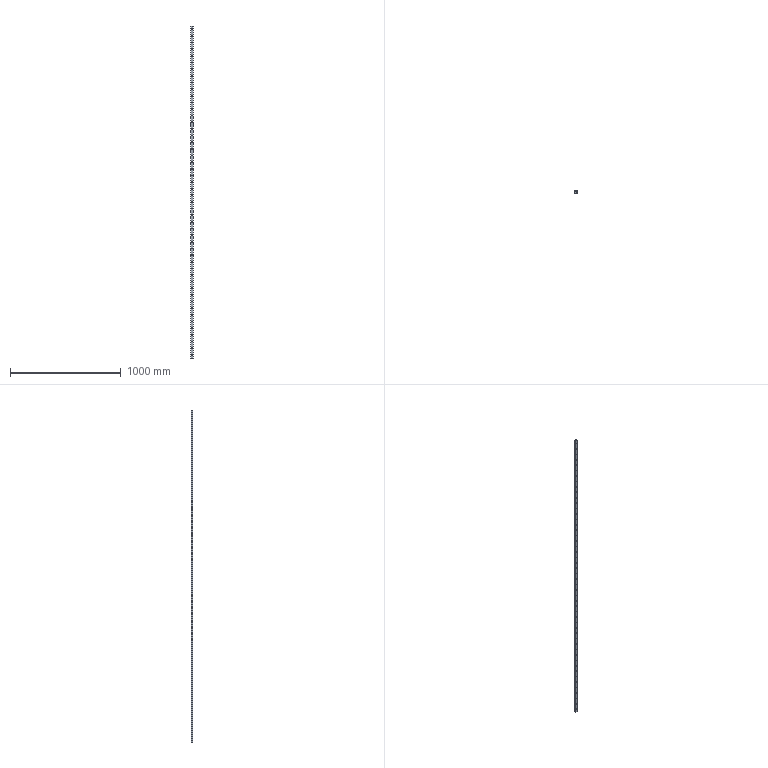Part | SolidWorks | features LocalLPattern 1, ReferencePattern 1 | 1 solid | 276 faces | box 20 x 17.5 x 3000 mm | volume 901599 mm3 | cylinder 206 | plane 70 | commonest cylinder face diameters 6 x100 9.5 x100 1.817 x6